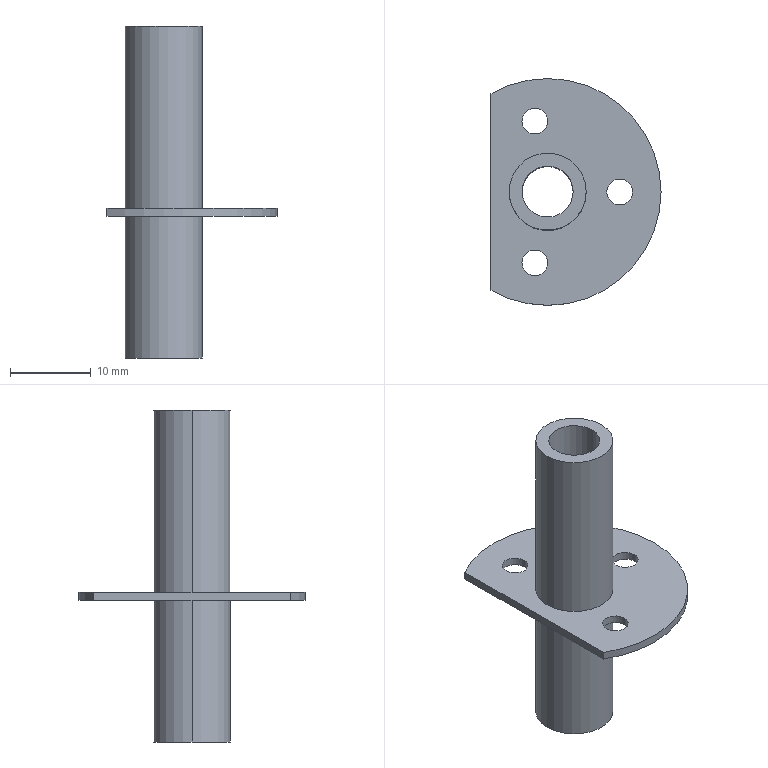Part | SolidWorks | features BaseBody 1 | 1 solid | 18 faces | box 21 x 28 x 41 mm | volume 2044 mm3 | cylinder 13 | plane 5 | commonest cylinder face diameters 3.175 x6 9.525 x4 6.3 x2 28 x1
STEP:
#1=CARTESIAN_POINT('',(3.15,0.,-17.5));
#2=VERTEX_POINT('',#1);
#3=CARTESIAN_POINT('',(-3.15,0.,-17.5));
#4=VERTEX_POINT('',#3);
#5=CARTESIAN_POINT('',(0.,0.,-17.5));
#6=DIRECTION('',(0.,0.,-1.));
#7=DIRECTION('',(1.,0.,0.));
#8=AXIS2_PLACEMENT_3D('',#5,#6,#7);
#9=CIRCLE('',#8,3.15);
#10=EDGE_CURVE('',#2,#4,#9,.T.);
#11=ORIENTED_EDGE('',*,*,#10,.T.);
#12=CARTESIAN_POINT('',(-3.15,0.,23.5));
#13=VERTEX_POINT('',#12);
#14=CARTESIAN_POINT('',(-3.15,0.,-17.5));
#15=DIRECTION('',(0.,0.,1.));
#16=VECTOR('',#15,1000.);
#17=LINE('',#14,#16);
#18=EDGE_CURVE('',#4,#13,#17,.T.);
#19=ORIENTED_EDGE('',*,*,#18,.T.);
#20=CARTESIAN_POINT('',(3.15,0.,23.5));
#21=VERTEX_POINT('',#20);
#22=CARTESIAN_POINT('',(0.,0.,23.5));
#23=DIRECTION('',(0.,0.,1.));
#24=DIRECTION('',(1.,0.,0.));
#25=AXIS2_PLACEMENT_3D('',#22,#23,#24);
#26=CIRCLE('',#25,3.15);
#27=EDGE_CURVE('',#13,#21,#26,.T.);
#28=ORIENTED_EDGE('',*,*,#27,.T.);
#29=CARTESIAN_POINT('',(3.15,0.,-17.5));
#30=DIRECTION('',(0.,0.,1.));
#31=VECTOR('',#30,1000.);
#32=LINE('',#29,#31);
#33=EDGE_CURVE('',#2,#21,#32,.T.);
#34=ORIENTED_EDGE('',*,*,#33,.F.);
#35=EDGE_LOOP('',(#11,#19,#28,#34));
#36=FACE_OUTER_BOUND('',#35,.T.);
#37=CARTESIAN_POINT('',(0.,0.,-17.5));
#38=DIRECTION('',(0.,0.,1.));
#39=DIRECTION('',(1.,0.,0.));
#40=AXIS2_PLACEMENT_3D('',#37,#38,#39);
#41=CYLINDRICAL_SURFACE('',#40,3.15);
#42=ADVANCED_FACE('',(#36),#41,.F.);
#43=CARTESIAN_POINT('',(-4.762,0.,1.));
#44=VERTEX_POINT('',#43);
#45=CARTESIAN_POINT('',(4.762,0.,1.));
#46=VERTEX_POINT('',#45);
#47=CARTESIAN_POINT('',(0.,0.,1.));
#48=DIRECTION('',(0.,0.,-1.));
#49=DIRECTION('',(1.,0.,0.));
#50=AXIS2_PLACEMENT_3D('',#47,#48,#49);
#51=CIRCLE('',#50,4.762);
#52=EDGE_CURVE('',#44,#46,#51,.T.);
#53=ORIENTED_EDGE('',*,*,#52,.F.);
#54=CARTESIAN_POINT('',(-4.762,0.,23.5));
#55=VERTEX_POINT('',#54);
#56=CARTESIAN_POINT('',(-4.762,0.,1.));
#57=DIRECTION('',(0.,0.,1.));
#58=VECTOR('',#57,1000.);
#59=LINE('',#56,#58);
#60=EDGE_CURVE('',#44,#55,#59,.T.);
#61=ORIENTED_EDGE('',*,*,#60,.T.);
#62=CARTESIAN_POINT('',(4.762,0.,23.5));
#63=VERTEX_POINT('',#62);
#64=CARTESIAN_POINT('',(0.,0.,23.5));
#65=DIRECTION('',(0.,0.,1.));
#66=DIRECTION('',(1.,0.,0.));
#67=AXIS2_PLACEMENT_3D('',#64,#65,#66);
#68=CIRCLE('',#67,4.762);
#69=EDGE_CURVE('',#63,#55,#68,.T.);
#70=ORIENTED_EDGE('',*,*,#69,.F.);
#71=CARTESIAN_POINT('',(4.762,0.,1.));
#72=DIRECTION('',(0.,0.,1.));
#73=VECTOR('',#72,1000.);
#74=LINE('',#71,#73);
#75=EDGE_CURVE('',#46,#63,#74,.T.);
#76=ORIENTED_EDGE('',*,*,#75,.F.);
#77=EDGE_LOOP('',(#53,#61,#70,#76));
#78=FACE_OUTER_BOUND('',#77,.T.);
#79=CARTESIAN_POINT('',(0.,0.,1.));
#80=DIRECTION('',(0.,0.,1.));
#81=DIRECTION('',(1.,0.,0.));
#82=AXIS2_PLACEMENT_3D('',#79,#80,#81);
#83=CYLINDRICAL_SURFACE('',#82,4.762);
#84=ADVANCED_FACE('',(#78),#83,.T.);
#85=CARTESIAN_POINT('',(4.762,0.,-17.5));
#86=VERTEX_POINT('',#85);
#87=CARTESIAN_POINT('',(-4.762,0.,-17.5));
#88=VERTEX_POINT('',#87);
#89=CARTESIAN_POINT('',(0.,0.,-17.5));
#90=DIRECTION('',(0.,0.,1.));
#91=DIRECTION('',(1.,0.,0.));
#92=AXIS2_PLACEMENT_3D('',#89,#90,#91);
#93=CIRCLE('',#92,4.762);
#94=EDGE_CURVE('',#86,#88,#93,.T.);
#95=ORIENTED_EDGE('',*,*,#94,.T.);
#96=CARTESIAN_POINT('',(-4.762,0.,0.));
#97=VERTEX_POINT('',#96);
#98=CARTESIAN_POINT('',(-4.762,0.,-17.5));
#99=DIRECTION('',(0.,0.,1.));
#100=VECTOR('',#99,1000.);
#101=LINE('',#98,#100);
#102=EDGE_CURVE('',#88,#97,#101,.T.);
#103=ORIENTED_EDGE('',*,*,#102,.T.);
#104=CARTESIAN_POINT('',(4.762,0.,0.));
#105=VERTEX_POINT('',#104);
#106=CARTESIAN_POINT('',(0.,0.,0.));
#107=DIRECTION('',(0.,0.,1.));
#108=DIRECTION('',(1.,0.,0.));
#109=AXIS2_PLACEMENT_3D('',#106,#107,#108);
#110=CIRCLE('',#109,4.762);
#111=EDGE_CURVE('',#105,#97,#110,.T.);
#112=ORIENTED_EDGE('',*,*,#111,.F.);
#113=CARTESIAN_POINT('',(4.762,0.,-17.5));
#114=DIRECTION('',(0.,0.,1.));
#115=VECTOR('',#114,1000.);
#116=LINE('',#113,#115);
#117=EDGE_CURVE('',#86,#105,#116,.T.);
#118=ORIENTED_EDGE('',*,*,#117,.F.);
#119=EDGE_LOOP('',(#95,#103,#112,#118));
#120=FACE_OUTER_BOUND('',#119,.T.);
#121=CARTESIAN_POINT('',(0.,0.,-17.5));
#122=DIRECTION('',(0.,0.,1.));
#123=DIRECTION('',(1.,0.,0.));
#124=AXIS2_PLACEMENT_3D('',#121,#122,#123);
#125=CYLINDRICAL_SURFACE('',#124,4.762);
#126=ADVANCED_FACE('',(#120),#125,.T.);
#127=CARTESIAN_POINT('',(10.478,0.,1.));
#128=VERTEX_POINT('',#127);
#129=CARTESIAN_POINT('',(7.302,0.,1.));
#130=VERTEX_POINT('',#129);
#131=CARTESIAN_POINT('',(8.89,0.,1.));
#132=DIRECTION('',(0.,0.,-1.));
#133=DIRECTION('',(-1.,0.,0.));
#134=AXIS2_PLACEMENT_3D('',#131,#132,#133);
#135=CIRCLE('',#134,1.588);
#136=EDGE_CURVE('',#128,#130,#135,.T.);
#137=ORIENTED_EDGE('',*,*,#136,.F.);
#138=CARTESIAN_POINT('',(10.478,0.,0.));
#139=VERTEX_POINT('',#138);
#140=CARTESIAN_POINT('',(10.478,0.,1.));
#141=DIRECTION('',(0.,0.,-1.));
#142=VECTOR('',#141,1000.);
#143=LINE('',#140,#142);
#144=EDGE_CURVE('',#128,#139,#143,.T.);
#145=ORIENTED_EDGE('',*,*,#144,.T.);
#146=CARTESIAN_POINT('',(7.302,0.,0.));
#147=VERTEX_POINT('',#146);
#148=CARTESIAN_POINT('',(8.89,0.,0.));
#149=DIRECTION('',(0.,0.,-1.));
#150=DIRECTION('',(-1.,0.,0.));
#151=AXIS2_PLACEMENT_3D('',#148,#149,#150);
#152=CIRCLE('',#151,1.588);
#153=EDGE_CURVE('',#139,#147,#152,.T.);
#154=ORIENTED_EDGE('',*,*,#153,.T.);
#155=CARTESIAN_POINT('',(7.302,0.,1.));
#156=DIRECTION('',(0.,0.,-1.));
#157=VECTOR('',#156,1000.);
#158=LINE('',#155,#157);
#159=EDGE_CURVE('',#130,#147,#158,.T.);
#160=ORIENTED_EDGE('',*,*,#159,.F.);
#161=EDGE_LOOP('',(#137,#145,#154,#160));
#162=FACE_OUTER_BOUND('',#161,.T.);
#163=CARTESIAN_POINT('',(8.89,0.,1.));
#164=DIRECTION('',(0.,0.,-1.));
#165=DIRECTION('',(-1.,0.,0.));
#166=AXIS2_PLACEMENT_3D('',#163,#164,#165);
#167=CYLINDRICAL_SURFACE('',#166,1.588);
#168=ADVANCED_FACE('',(#162),#167,.F.);
#169=CARTESIAN_POINT('',(0.,8.747,1.));
#170=VERTEX_POINT('',#169);
#171=CARTESIAN_POINT('',(-3.175,8.747,1.));
#172=VERTEX_POINT('',#171);
#173=CARTESIAN_POINT('',(-1.587,8.747,1.));
#174=DIRECTION('',(0.,0.,-1.));
#175=DIRECTION('',(-1.,0.,0.));
#176=AXIS2_PLACEMENT_3D('',#173,#174,#175);
#177=CIRCLE('',#176,1.587);
#178=EDGE_CURVE('',#170,#172,#177,.T.);
#179=ORIENTED_EDGE('',*,*,#178,.F.);
#180=CARTESIAN_POINT('',(0.,8.747,0.));
#181=VERTEX_POINT('',#180);
#182=CARTESIAN_POINT('',(0.,8.747,1.));
#183=DIRECTION('',(0.,0.,-1.));
#184=VECTOR('',#183,1000.);
#185=LINE('',#182,#184);
#186=EDGE_CURVE('',#170,#181,#185,.T.);
#187=ORIENTED_EDGE('',*,*,#186,.T.);
#188=CARTESIAN_POINT('',(-3.175,8.747,0.));
#189=VERTEX_POINT('',#188);
#190=CARTESIAN_POINT('',(-1.587,8.747,0.));
#191=DIRECTION('',(0.,0.,-1.));
#192=DIRECTION('',(-1.,0.,0.));
#193=AXIS2_PLACEMENT_3D('',#190,#191,#192);
#194=CIRCLE('',#193,1.587);
#195=EDGE_CURVE('',#181,#189,#194,.T.);
#196=ORIENTED_EDGE('',*,*,#195,.T.);
#197=CARTESIAN_POINT('',(-3.175,8.747,1.));
#198=DIRECTION('',(0.,0.,-1.));
#199=VECTOR('',#198,1000.);
#200=LINE('',#197,#199);
#201=EDGE_CURVE('',#172,#189,#200,.T.);
#202=ORIENTED_EDGE('',*,*,#201,.F.);
#203=EDGE_LOOP('',(#179,#187,#196,#202));
#204=FACE_OUTER_BOUND('',#203,.T.);
#205=CARTESIAN_POINT('',(-1.587,8.747,1.));
#206=DIRECTION('',(0.,0.,-1.));
#207=DIRECTION('',(-1.,0.,0.));
#208=AXIS2_PLACEMENT_3D('',#205,#206,#207);
#209=CYLINDRICAL_SURFACE('',#208,1.587);
#210=ADVANCED_FACE('',(#204),#209,.F.);
#211=CARTESIAN_POINT('',(0.,-8.747,1.));
#212=VERTEX_POINT('',#211);
#213=CARTESIAN_POINT('',(-3.175,-8.747,1.));
#214=VERTEX_POINT('',#213);
#215=CARTESIAN_POINT('',(-1.587,-8.747,1.));
#216=DIRECTION('',(0.,0.,-1.));
#217=DIRECTION('',(-1.,0.,0.));
#218=AXIS2_PLACEMENT_3D('',#215,#216,#217);
#219=CIRCLE('',#218,1.587);
#220=EDGE_CURVE('',#212,#214,#219,.T.);
#221=ORIENTED_EDGE('',*,*,#220,.F.);
#222=CARTESIAN_POINT('',(0.,-8.747,0.));
#223=VERTEX_POINT('',#222);
#224=CARTESIAN_POINT('',(0.,-8.747,1.));
#225=DIRECTION('',(0.,0.,-1.));
#226=VECTOR('',#225,1000.);
#227=LINE('',#224,#226);
#228=EDGE_CURVE('',#212,#223,#227,.T.);
#229=ORIENTED_EDGE('',*,*,#228,.T.);
#230=CARTESIAN_POINT('',(-3.175,-8.747,0.));
#231=VERTEX_POINT('',#230);
#232=CARTESIAN_POINT('',(-1.587,-8.747,0.));
#233=DIRECTION('',(0.,0.,-1.));
#234=DIRECTION('',(-1.,0.,0.));
#235=AXIS2_PLACEMENT_3D('',#232,#233,#234);
#236=CIRCLE('',#235,1.587);
#237=EDGE_CURVE('',#223,#231,#236,.T.);
#238=ORIENTED_EDGE('',*,*,#237,.T.);
#239=CARTESIAN_POINT('',(-3.175,-8.747,1.));
#240=DIRECTION('',(0.,0.,-1.));
#241=VECTOR('',#240,1000.);
#242=LINE('',#239,#241);
#243=EDGE_CURVE('',#214,#231,#242,.T.);
#244=ORIENTED_EDGE('',*,*,#243,.F.);
#245=EDGE_LOOP('',(#221,#229,#238,#244));
#246=FACE_OUTER_BOUND('',#245,.T.);
#247=CARTESIAN_POINT('',(-1.587,-8.747,1.));
#248=DIRECTION('',(0.,0.,-1.));
#249=DIRECTION('',(-1.,0.,0.));
#250=AXIS2_PLACEMENT_3D('',#247,#248,#249);
#251=CYLINDRICAL_SURFACE('',#250,1.587);
#252=ADVANCED_FACE('',(#246),#251,.F.);
#253=ORIENTED_EDGE('',*,*,#18,.F.);
#254=CARTESIAN_POINT('',(0.,0.,-17.5));
#255=DIRECTION('',(0.,0.,-1.));
#256=DIRECTION('',(1.,0.,0.));
#257=AXIS2_PLACEMENT_3D('',#254,#255,#256);
#258=CIRCLE('',#257,3.15);
#259=EDGE_CURVE('',#4,#2,#258,.T.);
#260=ORIENTED_EDGE('',*,*,#259,.T.);
#261=ORIENTED_EDGE('',*,*,#33,.T.);
#262=CARTESIAN_POINT('',(0.,0.,23.5));
#263=DIRECTION('',(0.,0.,1.));
#264=DIRECTION('',(1.,0.,0.));
#265=AXIS2_PLACEMENT_3D('',#262,#263,#264);
#266=CIRCLE('',#265,3.15);
#267=EDGE_CURVE('',#21,#13,#266,.T.);
#268=ORIENTED_EDGE('',*,*,#267,.T.);
#269=EDGE_LOOP('',(#253,#260,#261,#268));
#270=FACE_OUTER_BOUND('',#269,.T.);
#271=CARTESIAN_POINT('',(0.,0.,-17.5));
#272=DIRECTION('',(0.,0.,1.));
#273=DIRECTION('',(1.,0.,0.));
#274=AXIS2_PLACEMENT_3D('',#271,#272,#273);
#275=CYLINDRICAL_SURFACE('',#274,3.15);
#276=ADVANCED_FACE('',(#270),#275,.F.);
#277=ORIENTED_EDGE('',*,*,#267,.F.);
#278=ORIENTED_EDGE('',*,*,#27,.F.);
#279=EDGE_LOOP('',(#277,#278));
#280=FACE_BOUND('',#279,.T.);
#281=ORIENTED_EDGE('',*,*,#69,.T.);
#282=CARTESIAN_POINT('',(0.,0.,23.5));
#283=DIRECTION('',(0.,0.,1.));
#284=DIRECTION('',(1.,0.,0.));
#285=AXIS2_PLACEMENT_3D('',#282,#283,#284);
#286=CIRCLE('',#285,4.762);
#287=EDGE_CURVE('',#55,#63,#286,.T.);
#288=ORIENTED_EDGE('',*,*,#287,.T.);
#289=EDGE_LOOP('',(#281,#288));
#290=FACE_OUTER_BOUND('',#289,.T.);
#291=CARTESIAN_POINT('',(-4.82,-4.82,23.5));
#292=DIRECTION('',(0.,0.,1.));
#293=DIRECTION('',(1.,0.,0.));
#294=AXIS2_PLACEMENT_3D('',#291,#292,#293);
#295=PLANE('',#294);
#296=ADVANCED_FACE('',(#280,#290),#295,.T.);
#297=ORIENTED_EDGE('',*,*,#10,.F.);
#298=ORIENTED_EDGE('',*,*,#259,.F.);
#299=EDGE_LOOP('',(#297,#298));
#300=FACE_BOUND('',#299,.T.);
#301=ORIENTED_EDGE('',*,*,#94,.F.);
#302=CARTESIAN_POINT('',(0.,0.,-17.5));
#303=DIRECTION('',(0.,0.,1.));
#304=DIRECTION('',(1.,0.,0.));
#305=AXIS2_PLACEMENT_3D('',#302,#303,#304);
#306=CIRCLE('',#305,4.762);
#307=EDGE_CURVE('',#88,#86,#306,.T.);
#308=ORIENTED_EDGE('',*,*,#307,.F.);
#309=EDGE_LOOP('',(#301,#308));
#310=FACE_OUTER_BOUND('',#309,.T.);
#311=CARTESIAN_POINT('',(-4.82,-4.82,-17.5));
#312=DIRECTION('',(0.,0.,1.));
#313=DIRECTION('',(1.,0.,0.));
#314=AXIS2_PLACEMENT_3D('',#311,#312,#313);
#315=PLANE('',#314);
#316=ADVANCED_FACE('',(#300,#310),#315,.F.);
#317=ORIENTED_EDGE('',*,*,#60,.F.);
#318=CARTESIAN_POINT('',(0.,0.,1.));
#319=DIRECTION('',(0.,0.,-1.));
#320=DIRECTION('',(1.,0.,0.));
#321=AXIS2_PLACEMENT_3D('',#318,#319,#320);
#322=CIRCLE('',#321,4.762);
#323=EDGE_CURVE('',#46,#44,#322,.T.);
#324=ORIENTED_EDGE('',*,*,#323,.F.);
#325=ORIENTED_EDGE('',*,*,#75,.T.);
#326=ORIENTED_EDGE('',*,*,#287,.F.);
#327=EDGE_LOOP('',(#317,#324,#325,#326));
#328=FACE_OUTER_BOUND('',#327,.T.);
#329=CARTESIAN_POINT('',(0.,0.,1.));
#330=DIRECTION('',(0.,0.,1.));
#331=DIRECTION('',(1.,0.,0.));
#332=AXIS2_PLACEMENT_3D('',#329,#330,#331);
#333=CYLINDRICAL_SURFACE('',#332,4.762);
#334=ADVANCED_FACE('',(#328),#333,.T.);
#335=ORIENTED_EDGE('',*,*,#102,.F.);
#336=ORIENTED_EDGE('',*,*,#307,.T.);
#337=ORIENTED_EDGE('',*,*,#117,.T.);
#338=CARTESIAN_POINT('',(0.,0.,0.));
#339=DIRECTION('',(0.,0.,1.));
#340=DIRECTION('',(1.,0.,0.));
#341=AXIS2_PLACEMENT_3D('',#338,#339,#340);
#342=CIRCLE('',#341,4.762);
#343=EDGE_CURVE('',#97,#105,#342,.T.);
#344=ORIENTED_EDGE('',*,*,#343,.F.);
#345=EDGE_LOOP('',(#335,#336,#337,#344));
#346=FACE_OUTER_BOUND('',#345,.T.);
#347=CARTESIAN_POINT('',(0.,0.,-17.5));
#348=DIRECTION('',(0.,0.,1.));
#349=DIRECTION('',(1.,0.,0.));
#350=AXIS2_PLACEMENT_3D('',#347,#348,#349);
#351=CYLINDRICAL_SURFACE('',#350,4.762);
#352=ADVANCED_FACE('',(#346),#351,.T.);
#353=CARTESIAN_POINT('',(8.89,0.,1.));
#354=DIRECTION('',(0.,0.,-1.));
#355=DIRECTION('',(-1.,0.,0.));
#356=AXIS2_PLACEMENT_3D('',#353,#354,#355);
#357=CIRCLE('',#356,1.588);
#358=EDGE_CURVE('',#130,#128,#357,.T.);
#359=ORIENTED_EDGE('',*,*,#358,.T.);
#360=ORIENTED_EDGE('',*,*,#136,.T.);
#361=EDGE_LOOP('',(#359,#360));
#362=FACE_BOUND('',#361,.T.);
#363=CARTESIAN_POINT('',(-1.587,8.747,1.));
#364=DIRECTION('',(0.,0.,-1.));
#365=DIRECTION('',(-1.,0.,0.));
#366=AXIS2_PLACEMENT_3D('',#363,#364,#365);
#367=CIRCLE('',#366,1.587);
#368=EDGE_CURVE('',#172,#170,#367,.T.);
#369=ORIENTED_EDGE('',*,*,#368,.T.);
#370=ORIENTED_EDGE('',*,*,#178,.T.);
#371=EDGE_LOOP('',(#369,#370));
#372=FACE_BOUND('',#371,.T.);
#373=ORIENTED_EDGE('',*,*,#323,.T.);
#374=ORIENTED_EDGE('',*,*,#52,.T.);
#375=EDGE_LOOP('',(#373,#374));
#376=FACE_BOUND('',#375,.T.);
#377=CARTESIAN_POINT('',(-1.587,-8.747,1.));
#378=DIRECTION('',(0.,0.,-1.));
#379=DIRECTION('',(-1.,0.,0.));
#380=AXIS2_PLACEMENT_3D('',#377,#378,#379);
#381=CIRCLE('',#380,1.587);
#382=EDGE_CURVE('',#214,#212,#381,.T.);
#383=ORIENTED_EDGE('',*,*,#382,.T.);
#384=ORIENTED_EDGE('',*,*,#220,.T.);
#385=EDGE_LOOP('',(#383,#384));
#386=FACE_BOUND('',#385,.T.);
#387=CARTESIAN_POINT('',(-7.,-12.124,1.));
#388=VERTEX_POINT('',#387);
#389=CARTESIAN_POINT('',(-7.,12.124,1.));
#390=VERTEX_POINT('',#389);
#391=CARTESIAN_POINT('',(0.,0.,1.));
#392=DIRECTION('',(0.,0.,1.));
#393=DIRECTION('',(-1.,0.,0.));
#394=AXIS2_PLACEMENT_3D('',#391,#392,#393);
#395=CIRCLE('',#394,14.);
#396=EDGE_CURVE('',#388,#390,#395,.T.);
#397=ORIENTED_EDGE('',*,*,#396,.T.);
#398=CARTESIAN_POINT('',(-7.,0.,1.));
#399=DIRECTION('',(0.,-1.,0.));
#400=VECTOR('',#399,1000.);
#401=LINE('',#398,#400);
#402=EDGE_CURVE('',#390,#388,#401,.T.);
#403=ORIENTED_EDGE('',*,*,#402,.T.);
#404=EDGE_LOOP('',(#397,#403));
#405=FACE_OUTER_BOUND('',#404,.T.);
#406=CARTESIAN_POINT('',(-7.,-14.168,1.));
#407=DIRECTION('',(0.,0.,1.));
#408=DIRECTION('',(1.,0.,0.));
#409=AXIS2_PLACEMENT_3D('',#406,#407,#408);
#410=PLANE('',#409);
#411=ADVANCED_FACE('',(#362,#372,#376,#386,#405),#410,.T.);
#412=CARTESIAN_POINT('',(8.89,0.,0.));
#413=DIRECTION('',(0.,0.,-1.));
#414=DIRECTION('',(-1.,0.,0.));
#415=AXIS2_PLACEMENT_3D('',#412,#413,#414);
#416=CIRCLE('',#415,1.588);
#417=EDGE_CURVE('',#147,#139,#416,.T.);
#418=ORIENTED_EDGE('',*,*,#417,.F.);
#419=ORIENTED_EDGE('',*,*,#153,.F.);
#420=EDGE_LOOP('',(#418,#419));
#421=FACE_BOUND('',#420,.T.);
#422=CARTESIAN_POINT('',(-1.587,8.747,0.));
#423=DIRECTION('',(0.,0.,-1.));
#424=DIRECTION('',(-1.,0.,0.));
#425=AXIS2_PLACEMENT_3D('',#422,#423,#424);
#426=CIRCLE('',#425,1.587);
#427=EDGE_CURVE('',#189,#181,#426,.T.);
#428=ORIENTED_EDGE('',*,*,#427,.F.);
#429=ORIENTED_EDGE('',*,*,#195,.F.);
#430=EDGE_LOOP('',(#428,#429));
#431=FACE_BOUND('',#430,.T.);
#432=ORIENTED_EDGE('',*,*,#111,.T.);
#433=ORIENTED_EDGE('',*,*,#343,.T.);
#434=EDGE_LOOP('',(#432,#433));
#435=FACE_BOUND('',#434,.T.);
#436=CARTESIAN_POINT('',(-1.587,-8.747,0.));
#437=DIRECTION('',(0.,0.,-1.));
#438=DIRECTION('',(-1.,0.,0.));
#439=AXIS2_PLACEMENT_3D('',#436,#437,#438);
#440=CIRCLE('',#439,1.587);
#441=EDGE_CURVE('',#231,#223,#440,.T.);
#442=ORIENTED_EDGE('',*,*,#441,.F.);
#443=ORIENTED_EDGE('',*,*,#237,.F.);
#444=EDGE_LOOP('',(#442,#443));
#445=FACE_BOUND('',#444,.T.);
#446=CARTESIAN_POINT('',(-7.,12.124,0.));
#447=VERTEX_POINT('',#446);
#448=CARTESIAN_POINT('',(-7.,-12.124,0.));
#449=VERTEX_POINT('',#448);
#450=CARTESIAN_POINT('',(-7.,0.,0.));
#451=DIRECTION('',(0.,-1.,0.));
#452=VECTOR('',#451,1000.);
#453=LINE('',#450,#452);
#454=EDGE_CURVE('',#447,#449,#453,.T.);
#455=ORIENTED_EDGE('',*,*,#454,.F.);
#456=CARTESIAN_POINT('',(0.,0.,0.));
#457=DIRECTION('',(0.,0.,1.));
#458=DIRECTION('',(-1.,0.,0.));
#459=AXIS2_PLACEMENT_3D('',#456,#457,#458);
#460=CIRCLE('',#459,14.);
#461=EDGE_CURVE('',#449,#447,#460,.T.);
#462=ORIENTED_EDGE('',*,*,#461,.F.);
#463=EDGE_LOOP('',(#455,#462));
#464=FACE_OUTER_BOUND('',#463,.T.);
#465=CARTESIAN_POINT('',(-7.,-14.168,0.));
#466=DIRECTION('',(0.,0.,1.));
#467=DIRECTION('',(1.,0.,0.));
#468=AXIS2_PLACEMENT_3D('',#465,#466,#467);
#469=PLANE('',#468);
#470=ADVANCED_FACE('',(#421,#431,#435,#445,#464),#469,.F.);
#471=ORIENTED_EDGE('',*,*,#144,.F.);
#472=ORIENTED_EDGE('',*,*,#358,.F.);
#473=ORIENTED_EDGE('',*,*,#159,.T.);
#474=ORIENTED_EDGE('',*,*,#417,.T.);
#475=EDGE_LOOP('',(#471,#472,#473,#474));
#476=FACE_OUTER_BOUND('',#475,.T.);
#477=CARTESIAN_POINT('',(8.89,0.,1.));
#478=DIRECTION('',(0.,0.,-1.));
#479=DIRECTION('',(-1.,0.,0.));
#480=AXIS2_PLACEMENT_3D('',#477,#478,#479);
#481=CYLINDRICAL_SURFACE('',#480,1.588);
#482=ADVANCED_FACE('',(#476),#481,.F.);
#483=ORIENTED_EDGE('',*,*,#186,.F.);
#484=ORIENTED_EDGE('',*,*,#368,.F.);
#485=ORIENTED_EDGE('',*,*,#201,.T.);
#486=ORIENTED_EDGE('',*,*,#427,.T.);
#487=EDGE_LOOP('',(#483,#484,#485,#486));
#488=FACE_OUTER_BOUND('',#487,.T.);
#489=CARTESIAN_POINT('',(-1.587,8.747,1.));
#490=DIRECTION('',(0.,0.,-1.));
#491=DIRECTION('',(-1.,0.,0.));
#492=AXIS2_PLACEMENT_3D('',#489,#490,#491);
#493=CYLINDRICAL_SURFACE('',#492,1.587);
#494=ADVANCED_FACE('',(#488),#493,.F.);
#495=ORIENTED_EDGE('',*,*,#228,.F.);
#496=ORIENTED_EDGE('',*,*,#382,.F.);
#497=ORIENTED_EDGE('',*,*,#243,.T.);
#498=ORIENTED_EDGE('',*,*,#441,.T.);
#499=EDGE_LOOP('',(#495,#496,#497,#498));
#500=FACE_OUTER_BOUND('',#499,.T.);
#501=CARTESIAN_POINT('',(-1.587,-8.747,1.));
#502=DIRECTION('',(0.,0.,-1.));
#503=DIRECTION('',(-1.,0.,0.));
#504=AXIS2_PLACEMENT_3D('',#501,#502,#503);
#505=CYLINDRICAL_SURFACE('',#504,1.587);
#506=ADVANCED_FACE('',(#500),#505,.F.);
#507=CARTESIAN_POINT('',(-7.,-12.124,0.5));
#508=DIRECTION('',(0.,0.,-1.));
#509=VECTOR('',#508,1000.);
#510=LINE('',#507,#509);
#511=EDGE_CURVE('',#388,#449,#510,.T.);
#512=ORIENTED_EDGE('',*,*,#511,.F.);
#513=ORIENTED_EDGE('',*,*,#402,.F.);
#514=CARTESIAN_POINT('',(-7.,12.124,0.5));
#515=DIRECTION('',(0.,0.,1.));
#516=VECTOR('',#515,1000.);
#517=LINE('',#514,#516);
#518=EDGE_CURVE('',#447,#390,#517,.T.);
#519=ORIENTED_EDGE('',*,*,#518,.F.);
#520=ORIENTED_EDGE('',*,*,#454,.T.);
#521=EDGE_LOOP('',(#512,#513,#519,#520));
#522=FACE_OUTER_BOUND('',#521,.T.);
#523=CARTESIAN_POINT('',(-7.,-12.124,1.));
#524=DIRECTION('',(1.,0.,0.));
#525=DIRECTION('',(0.,0.,-1.));
#526=AXIS2_PLACEMENT_3D('',#523,#524,#525);
#527=PLANE('',#526);
#528=ADVANCED_FACE('',(#522),#527,.F.);
#529=ORIENTED_EDGE('',*,*,#518,.T.);
#530=ORIENTED_EDGE('',*,*,#396,.F.);
#531=ORIENTED_EDGE('',*,*,#511,.T.);
#532=ORIENTED_EDGE('',*,*,#461,.T.);
#533=EDGE_LOOP('',(#529,#530,#531,#532));
#534=FACE_OUTER_BOUND('',#533,.T.);
#535=CARTESIAN_POINT('',(0.,0.,1.));
#536=DIRECTION('',(0.,0.,-1.));
#537=DIRECTION('',(-1.,0.,0.));
#538=AXIS2_PLACEMENT_3D('',#535,#536,#537);
#539=CYLINDRICAL_SURFACE('',#538,14.);
#540=ADVANCED_FACE('',(#534),#539,.T.);
#541=CLOSED_SHELL('',(#42,#84,#126,#168,#210,#252,#276,#296,#316,#334,#352,#411,#470,#482,#494,#506,#528,#540));
#542=MANIFOLD_SOLID_BREP('',#541);
#543=CARTESIAN_POINT('',(0.,0.,0.));
#544=DIRECTION('',(0.,0.,1.));
#545=DIRECTION('',(1.,0.,0.));
#546=AXIS2_PLACEMENT_3D('',#543,#544,#545);
#547=(LENGTH_UNIT()NAMED_UNIT(*)SI_UNIT(.MILLI.,.METRE.));
#548=UNCERTAINTY_MEASURE_WITH_UNIT(LENGTH_MEASURE(0.00001),#547,'','');
#549=(NAMED_UNIT(*)PLANE_ANGLE_UNIT()SI_UNIT($,.RADIAN.));
#550=(NAMED_UNIT(*)SI_UNIT($,.STERADIAN.)SOLID_ANGLE_UNIT());
#551=(GEOMETRIC_REPRESENTATION_CONTEXT(3)GLOBAL_UNCERTAINTY_ASSIGNED_CONTEXT((#548))GLOBAL_UNIT_ASSIGNED_CONTEXT((#547,#549,#550))REPRESENTATION_CONTEXT('',''));
#552=ADVANCED_BREP_SHAPE_REPRESENTATION('',(#542,#546),#551);